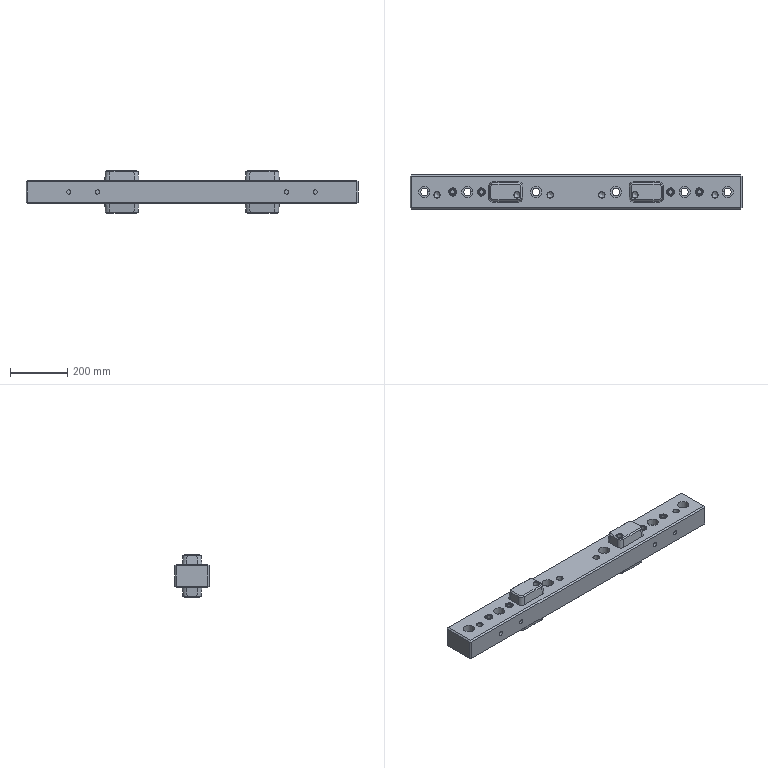Part | STEP file | solid 128 | 1 solid | 178 faces | box 1159 x 120 x 150 mm | volume 11583265 mm3 | plane 84 | cylinder 50 | cone 20 | spline 16 | torus 8 | commonest cylinder face diameters 15 x16 30 x16 21 x6 26 x6 39 x6